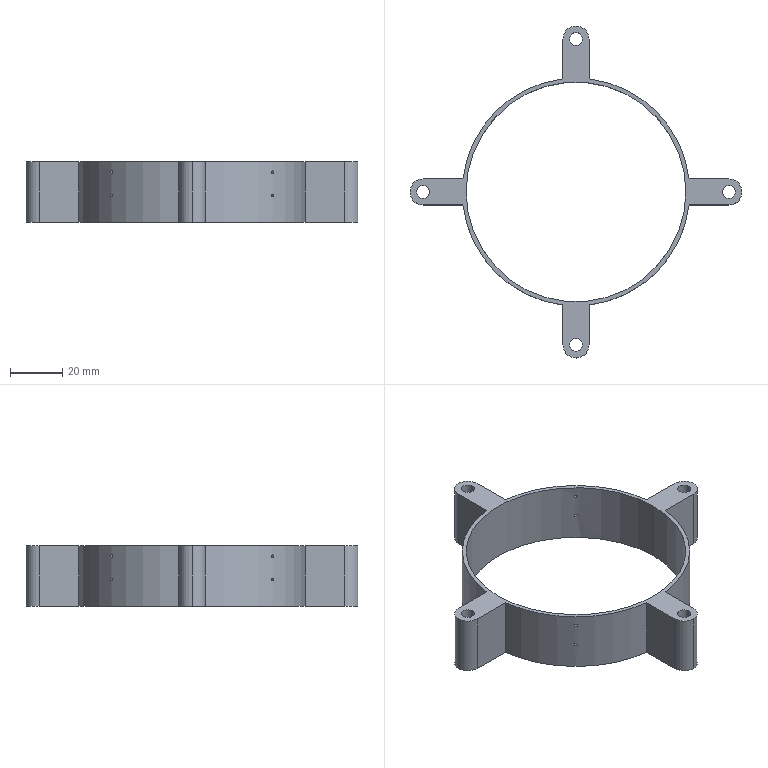Part | SolidWorks | features ICE 3, CirPattern 2, Extrusion 1, Fillet 1 | 1 solid | 48 faces | box 127.2 x 127.2 x 23.3 mm | volume 25300 mm3 | cylinder 38 | plane 10 | commonest cylinder face diameters 1 x16 5 x8 10 x8 87.2 x4 84.2 x2